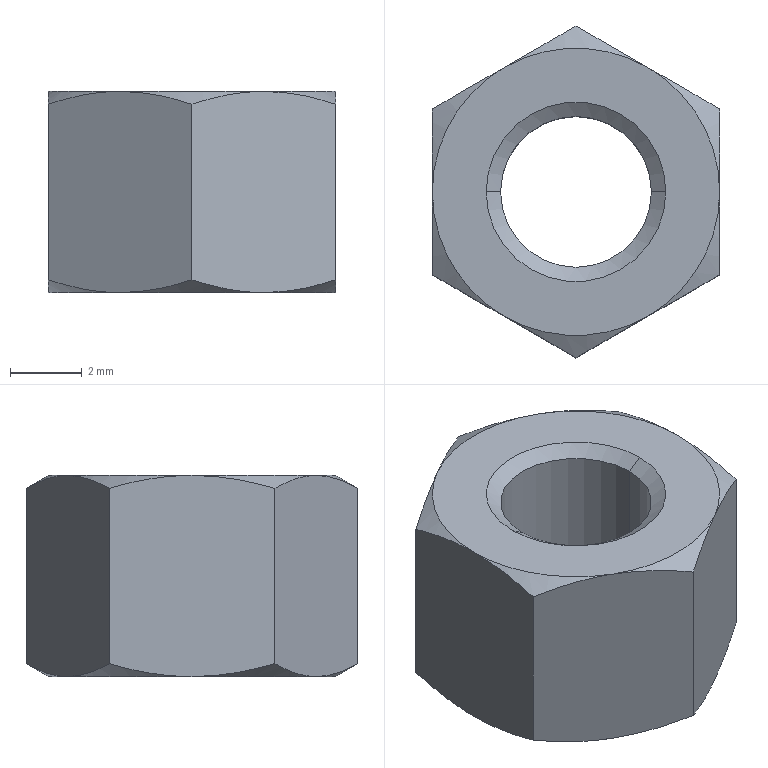Part | SolidWorks | features RevCut 3, Extrusion 1, LPattern 1 | 1 solid | 28 faces | box 8 x 9.238 x 5.6 mm | volume 229.964 mm3 | cone 16 | plane 8 | cylinder 4 | commonest cylinder face diameters 4.2 x2 5 x2
STEP:
#1=CARTESIAN_POINT('',(-2.5,0.,-5.6));
#2=VERTEX_POINT('',#1);
#3=CARTESIAN_POINT('',(2.5,0.,-5.6));
#4=VERTEX_POINT('',#3);
#5=CARTESIAN_POINT('',(0.,0.,-5.6));
#6=DIRECTION('',(0.,0.,1.));
#7=DIRECTION('',(-1.,0.,0.));
#8=AXIS2_PLACEMENT_3D('',#5,#6,#7);
#9=CIRCLE('',#8,2.5);
#10=EDGE_CURVE('',#2,#4,#9,.T.);
#11=ORIENTED_EDGE('',*,*,#10,.F.);
#12=CARTESIAN_POINT('',(-2.5,0.,-5.575));
#13=VERTEX_POINT('',#12);
#14=CARTESIAN_POINT('',(-2.5,0.,-25.038));
#15=DIRECTION('',(0.,0.,1.));
#16=VECTOR('',#15,1000.);
#17=LINE('',#14,#16);
#18=EDGE_CURVE('',#2,#13,#17,.T.);
#19=ORIENTED_EDGE('',*,*,#18,.T.);
#20=CARTESIAN_POINT('',(2.5,0.,-5.575));
#21=VERTEX_POINT('',#20);
#22=CARTESIAN_POINT('',(0.,0.,-5.575));
#23=DIRECTION('',(0.,0.,1.));
#24=DIRECTION('',(1.,0.,0.));
#25=AXIS2_PLACEMENT_3D('',#22,#23,#24);
#26=CIRCLE('',#25,2.5);
#27=EDGE_CURVE('',#13,#21,#26,.T.);
#28=ORIENTED_EDGE('',*,*,#27,.T.);
#29=CARTESIAN_POINT('',(2.5,0.,-25.038));
#30=DIRECTION('',(0.,0.,1.));
#31=VECTOR('',#30,1000.);
#32=LINE('',#29,#31);
#33=EDGE_CURVE('',#4,#21,#32,.T.);
#34=ORIENTED_EDGE('',*,*,#33,.F.);
#35=EDGE_LOOP('',(#11,#19,#28,#34));
#36=FACE_OUTER_BOUND('',#35,.T.);
#37=CARTESIAN_POINT('',(0.,0.,-25.038));
#38=DIRECTION('',(0.,0.,1.));
#39=DIRECTION('',(1.,0.,0.));
#40=AXIS2_PLACEMENT_3D('',#37,#38,#39);
#41=CYLINDRICAL_SURFACE('',#40,2.5);
#42=ADVANCED_FACE('',(#36),#41,.F.);
#43=CARTESIAN_POINT('',(-2.1,0.,-5.295));
#44=VERTEX_POINT('',#43);
#45=CARTESIAN_POINT('',(2.1,0.,-5.295));
#46=VERTEX_POINT('',#45);
#47=CARTESIAN_POINT('',(0.,0.,-5.295));
#48=DIRECTION('',(0.,0.,1.));
#49=DIRECTION('',(-1.,0.,0.));
#50=AXIS2_PLACEMENT_3D('',#47,#48,#49);
#51=CIRCLE('',#50,2.1);
#52=EDGE_CURVE('',#44,#46,#51,.T.);
#53=ORIENTED_EDGE('',*,*,#52,.T.);
#54=CARTESIAN_POINT('',(2.5,0.,-5.575));
#55=DIRECTION('',(0.8192,0.,-0.5736));
#56=VECTOR('',#55,1000.);
#57=LINE('',#54,#56);
#58=EDGE_CURVE('',#46,#21,#57,.T.);
#59=ORIENTED_EDGE('',*,*,#58,.T.);
#60=ORIENTED_EDGE('',*,*,#27,.F.);
#61=CARTESIAN_POINT('',(-2.5,0.,-5.575));
#62=DIRECTION('',(-0.8192,0.,-0.5736));
#63=VECTOR('',#62,1000.);
#64=LINE('',#61,#63);
#65=EDGE_CURVE('',#44,#13,#64,.T.);
#66=ORIENTED_EDGE('',*,*,#65,.F.);
#67=EDGE_LOOP('',(#53,#59,#60,#66));
#68=FACE_OUTER_BOUND('',#67,.T.);
#69=CARTESIAN_POINT('',(0.,0.,-5.575));
#70=DIRECTION('',(0.,0.,-1.));
#71=DIRECTION('',(-1.,0.,0.));
#72=AXIS2_PLACEMENT_3D('',#69,#70,#71);
#73=CONICAL_SURFACE('',#72,2.5,0.9599);
#74=ADVANCED_FACE('',(#68),#73,.F.);
#75=CARTESIAN_POINT('',(2.1,0.,-0.2801));
#76=VERTEX_POINT('',#75);
#77=CARTESIAN_POINT('',(-2.1,0.,-0.2801));
#78=VERTEX_POINT('',#77);
#79=CARTESIAN_POINT('',(0.,0.,-0.2801));
#80=DIRECTION('',(0.,0.,-1.));
#81=DIRECTION('',(1.,0.,0.));
#82=AXIS2_PLACEMENT_3D('',#79,#80,#81);
#83=CIRCLE('',#82,2.1);
#84=EDGE_CURVE('',#76,#78,#83,.T.);
#85=ORIENTED_EDGE('',*,*,#84,.T.);
#86=CARTESIAN_POINT('',(-2.5,0.,0.));
#87=VERTEX_POINT('',#86);
#88=CARTESIAN_POINT('',(-2.06,0.,-0.3081));
#89=DIRECTION('',(-0.8192,0.,0.5736));
#90=VECTOR('',#89,1000.);
#91=LINE('',#88,#90);
#92=EDGE_CURVE('',#78,#87,#91,.T.);
#93=ORIENTED_EDGE('',*,*,#92,.T.);
#94=CARTESIAN_POINT('',(2.5,0.,0.));
#95=VERTEX_POINT('',#94);
#96=CARTESIAN_POINT('',(0.,0.,0.));
#97=DIRECTION('',(0.,0.,1.));
#98=DIRECTION('',(1.,0.,0.));
#99=AXIS2_PLACEMENT_3D('',#96,#97,#98);
#100=CIRCLE('',#99,2.5);
#101=EDGE_CURVE('',#87,#95,#100,.T.);
#102=ORIENTED_EDGE('',*,*,#101,.T.);
#103=CARTESIAN_POINT('',(2.06,0.,-0.3081));
#104=DIRECTION('',(0.8192,0.,0.5736));
#105=VECTOR('',#104,1000.);
#106=LINE('',#103,#105);
#107=EDGE_CURVE('',#76,#95,#106,.T.);
#108=ORIENTED_EDGE('',*,*,#107,.F.);
#109=EDGE_LOOP('',(#85,#93,#102,#108));
#110=FACE_OUTER_BOUND('',#109,.T.);
#111=CARTESIAN_POINT('',(0.,0.,-0.3081));
#112=DIRECTION('',(0.,0.,1.));
#113=DIRECTION('',(1.,0.,0.));
#114=AXIS2_PLACEMENT_3D('',#111,#112,#113);
#115=CONICAL_SURFACE('',#114,2.06,0.9599);
#116=ADVANCED_FACE('',(#110),#115,.F.);
#117=ORIENTED_EDGE('',*,*,#52,.F.);
#118=CARTESIAN_POINT('',(-2.1,0.,-5.6));
#119=DIRECTION('',(0.,0.,1.));
#120=VECTOR('',#119,1000.);
#121=LINE('',#118,#120);
#122=EDGE_CURVE('',#44,#78,#121,.T.);
#123=ORIENTED_EDGE('',*,*,#122,.T.);
#124=ORIENTED_EDGE('',*,*,#84,.F.);
#125=CARTESIAN_POINT('',(2.1,0.,-5.6));
#126=DIRECTION('',(0.,0.,1.));
#127=VECTOR('',#126,1000.);
#128=LINE('',#125,#127);
#129=EDGE_CURVE('',#46,#76,#128,.T.);
#130=ORIENTED_EDGE('',*,*,#129,.F.);
#131=EDGE_LOOP('',(#117,#123,#124,#130));
#132=FACE_OUTER_BOUND('',#131,.T.);
#133=CARTESIAN_POINT('',(0.,0.,-5.6));
#134=DIRECTION('',(0.,0.,1.));
#135=DIRECTION('',(1.,0.,0.));
#136=AXIS2_PLACEMENT_3D('',#133,#134,#135);
#137=CYLINDRICAL_SURFACE('',#136,2.1);
#138=ADVANCED_FACE('',(#132),#137,.F.);
#139=ORIENTED_EDGE('',*,*,#122,.F.);
#140=CARTESIAN_POINT('',(0.,0.,-5.295));
#141=DIRECTION('',(0.,0.,1.));
#142=DIRECTION('',(-1.,0.,0.));
#143=AXIS2_PLACEMENT_3D('',#140,#141,#142);
#144=CIRCLE('',#143,2.1);
#145=EDGE_CURVE('',#46,#44,#144,.T.);
#146=ORIENTED_EDGE('',*,*,#145,.F.);
#147=ORIENTED_EDGE('',*,*,#129,.T.);
#148=CARTESIAN_POINT('',(0.,0.,-0.2801));
#149=DIRECTION('',(0.,0.,-1.));
#150=DIRECTION('',(1.,0.,0.));
#151=AXIS2_PLACEMENT_3D('',#148,#149,#150);
#152=CIRCLE('',#151,2.1);
#153=EDGE_CURVE('',#78,#76,#152,.T.);
#154=ORIENTED_EDGE('',*,*,#153,.F.);
#155=EDGE_LOOP('',(#139,#146,#147,#154));
#156=FACE_OUTER_BOUND('',#155,.T.);
#157=CARTESIAN_POINT('',(0.,0.,-5.6));
#158=DIRECTION('',(0.,0.,1.));
#159=DIRECTION('',(1.,0.,0.));
#160=AXIS2_PLACEMENT_3D('',#157,#158,#159);
#161=CYLINDRICAL_SURFACE('',#160,2.1);
#162=ADVANCED_FACE('',(#156),#161,.F.);
#163=CARTESIAN_POINT('',(-4.,2.309,-5.243));
#164=VERTEX_POINT('',#163);
#165=CARTESIAN_POINT('',(-4.,2.309,-0.3573));
#166=VERTEX_POINT('',#165);
#167=CARTESIAN_POINT('',(-4.,2.309,-5.6));
#168=DIRECTION('',(0.,0.,1.));
#169=VECTOR('',#168,1000.);
#170=LINE('',#167,#169);
#171=EDGE_CURVE('',#164,#166,#170,.T.);
#172=ORIENTED_EDGE('',*,*,#171,.T.);
#173=CARTESIAN_POINT('',(-2.,3.464,0.));
#174=VERTEX_POINT('',#173);
#175=CARTESIAN_POINT('',(-4.,2.309,-0.3573));
#176=CARTESIAN_POINT('',(-3.346,2.687,-0.1392));
#177=CARTESIAN_POINT('',(-2.681,3.071,0.));
#178=CARTESIAN_POINT('',(-2.,3.464,0.));
#179=B_SPLINE_CURVE_WITH_KNOTS('',3,(#175,#176,#177,#178),.UNSPECIFIED.,.F.,.F.,(4,4),(0.000000238,0.002337),.UNSPECIFIED.);
#180=EDGE_CURVE('',#166,#174,#179,.T.);
#181=ORIENTED_EDGE('',*,*,#180,.T.);
#182=CARTESIAN_POINT('',(0.,4.619,-0.3573));
#183=VERTEX_POINT('',#182);
#184=CARTESIAN_POINT('',(-2.,3.464,0.));
#185=CARTESIAN_POINT('',(-1.661,3.66,0.));
#186=CARTESIAN_POINT('',(-1.322,3.856,-0.03421));
#187=CARTESIAN_POINT('',(-0.6554,4.24,-0.1587));
#188=CARTESIAN_POINT('',(-0.3264,4.43,-0.2485));
#189=CARTESIAN_POINT('',(0.,4.619,-0.3573));
#190=B_SPLINE_CURVE_WITH_KNOTS('',3,(#184,#185,#186,#187,#188,#189),.UNSPECIFIED.,.F.,.F.,(4,2,4),(0.002337,0.003501,0.004665),.UNSPECIFIED.);
#191=EDGE_CURVE('',#174,#183,#190,.T.);
#192=ORIENTED_EDGE('',*,*,#191,.T.);
#193=CARTESIAN_POINT('',(0.,4.619,-5.243));
#194=VERTEX_POINT('',#193);
#195=CARTESIAN_POINT('',(0.,4.619,-5.6));
#196=DIRECTION('',(0.,0.,1.));
#197=VECTOR('',#196,1000.);
#198=LINE('',#195,#197);
#199=EDGE_CURVE('',#194,#183,#198,.T.);
#200=ORIENTED_EDGE('',*,*,#199,.F.);
#201=CARTESIAN_POINT('',(-2.,3.464,-5.6));
#202=VERTEX_POINT('',#201);
#203=CARTESIAN_POINT('',(-2.,3.464,-5.6));
#204=CARTESIAN_POINT('',(-1.661,3.66,-5.6));
#205=CARTESIAN_POINT('',(-1.322,3.856,-5.566));
#206=CARTESIAN_POINT('',(-0.6554,4.24,-5.441));
#207=CARTESIAN_POINT('',(-0.3264,4.43,-5.352));
#208=CARTESIAN_POINT('',(0.,4.619,-5.243));
#209=B_SPLINE_CURVE_WITH_KNOTS('',3,(#203,#204,#205,#206,#207,#208),.UNSPECIFIED.,.F.,.F.,(4,2,4),(0.002337,0.003501,0.004665),.UNSPECIFIED.);
#210=EDGE_CURVE('',#202,#194,#209,.T.);
#211=ORIENTED_EDGE('',*,*,#210,.F.);
#212=CARTESIAN_POINT('',(-4.,2.309,-5.243));
#213=CARTESIAN_POINT('',(-3.346,2.687,-5.461));
#214=CARTESIAN_POINT('',(-2.681,3.071,-5.6));
#215=CARTESIAN_POINT('',(-2.,3.464,-5.6));
#216=B_SPLINE_CURVE_WITH_KNOTS('',3,(#212,#213,#214,#215),.UNSPECIFIED.,.F.,.F.,(4,4),(0.000000238,0.002337),.UNSPECIFIED.);
#217=EDGE_CURVE('',#164,#202,#216,.T.);
#218=ORIENTED_EDGE('',*,*,#217,.F.);
#219=EDGE_LOOP('',(#172,#181,#192,#200,#211,#218));
#220=FACE_OUTER_BOUND('',#219,.T.);
#221=CARTESIAN_POINT('',(0.,4.619,-5.6));
#222=DIRECTION('',(-0.5,0.866,0.));
#223=DIRECTION('',(-0.866,-0.5,0.));
#224=AXIS2_PLACEMENT_3D('',#221,#222,#223);
#225=PLANE('',#224);
#226=ADVANCED_FACE('',(#220),#225,.T.);
#227=ORIENTED_EDGE('',*,*,#199,.T.);
#228=CARTESIAN_POINT('',(2.,3.464,0.));
#229=VERTEX_POINT('',#228);
#230=CARTESIAN_POINT('',(0.,4.619,-0.3573));
#231=CARTESIAN_POINT('',(0.6543,4.241,-0.1392));
#232=CARTESIAN_POINT('',(1.319,3.858,0.));
#233=CARTESIAN_POINT('',(2.,3.464,0.));
#234=B_SPLINE_CURVE_WITH_KNOTS('',3,(#230,#231,#232,#233),.UNSPECIFIED.,.F.,.F.,(4,4),(0.000000238,0.002337),.UNSPECIFIED.);
#235=EDGE_CURVE('',#183,#229,#234,.T.);
#236=ORIENTED_EDGE('',*,*,#235,.T.);
#237=CARTESIAN_POINT('',(4.,2.309,-0.3573));
#238=VERTEX_POINT('',#237);
#239=CARTESIAN_POINT('',(2.,3.464,0.));
#240=CARTESIAN_POINT('',(2.339,3.268,0.));
#241=CARTESIAN_POINT('',(2.678,3.072,-0.03421));
#242=CARTESIAN_POINT('',(3.345,2.688,-0.1587));
#243=CARTESIAN_POINT('',(3.674,2.498,-0.2485));
#244=CARTESIAN_POINT('',(4.,2.309,-0.3573));
#245=B_SPLINE_CURVE_WITH_KNOTS('',3,(#239,#240,#241,#242,#243,#244),.UNSPECIFIED.,.F.,.F.,(4,2,4),(0.002337,0.003501,0.004665),.UNSPECIFIED.);
#246=EDGE_CURVE('',#229,#238,#245,.T.);
#247=ORIENTED_EDGE('',*,*,#246,.T.);
#248=CARTESIAN_POINT('',(4.,2.309,-5.243));
#249=VERTEX_POINT('',#248);
#250=CARTESIAN_POINT('',(4.,2.309,-5.6));
#251=DIRECTION('',(0.,0.,1.));
#252=VECTOR('',#251,1000.);
#253=LINE('',#250,#252);
#254=EDGE_CURVE('',#249,#238,#253,.T.);
#255=ORIENTED_EDGE('',*,*,#254,.F.);
#256=CARTESIAN_POINT('',(2.,3.464,-5.6));
#257=VERTEX_POINT('',#256);
#258=CARTESIAN_POINT('',(2.,3.464,-5.6));
#259=CARTESIAN_POINT('',(2.339,3.268,-5.6));
#260=CARTESIAN_POINT('',(2.678,3.072,-5.566));
#261=CARTESIAN_POINT('',(3.345,2.688,-5.441));
#262=CARTESIAN_POINT('',(3.674,2.498,-5.352));
#263=CARTESIAN_POINT('',(4.,2.309,-5.243));
#264=B_SPLINE_CURVE_WITH_KNOTS('',3,(#258,#259,#260,#261,#262,#263),.UNSPECIFIED.,.F.,.F.,(4,2,4),(0.002337,0.003501,0.004665),.UNSPECIFIED.);
#265=EDGE_CURVE('',#257,#249,#264,.T.);
#266=ORIENTED_EDGE('',*,*,#265,.F.);
#267=CARTESIAN_POINT('',(0.,4.619,-5.243));
#268=CARTESIAN_POINT('',(0.6543,4.241,-5.461));
#269=CARTESIAN_POINT('',(1.319,3.858,-5.6));
#270=CARTESIAN_POINT('',(2.,3.464,-5.6));
#271=B_SPLINE_CURVE_WITH_KNOTS('',3,(#267,#268,#269,#270),.UNSPECIFIED.,.F.,.F.,(4,4),(0.000000238,0.002337),.UNSPECIFIED.);
#272=EDGE_CURVE('',#194,#257,#271,.T.);
#273=ORIENTED_EDGE('',*,*,#272,.F.);
#274=EDGE_LOOP('',(#227,#236,#247,#255,#266,#273));
#275=FACE_OUTER_BOUND('',#274,.T.);
#276=CARTESIAN_POINT('',(4.,2.309,-5.6));
#277=DIRECTION('',(0.5,0.866,0.));
#278=DIRECTION('',(-0.866,0.5,0.));
#279=AXIS2_PLACEMENT_3D('',#276,#277,#278);
#280=PLANE('',#279);
#281=ADVANCED_FACE('',(#275),#280,.T.);
#282=CARTESIAN_POINT('',(4.,-2.309,-0.3573));
#283=VERTEX_POINT('',#282);
#284=CARTESIAN_POINT('',(4.,0.,0.));
#285=VERTEX_POINT('',#284);
#286=CARTESIAN_POINT('',(4.,-2.309,-0.3573));
#287=CARTESIAN_POINT('',(4.,-1.934,-0.2488));
#288=CARTESIAN_POINT('',(4.,-1.549,-0.1579));
#289=CARTESIAN_POINT('',(4.,-0.778,-0.03354));
#290=CARTESIAN_POINT('',(4.,-0.3903,0.));
#291=CARTESIAN_POINT('',(4.,0.,0.));
#292=B_SPLINE_CURVE_WITH_KNOTS('',3,(#286,#287,#288,#289,#290,#291),.UNSPECIFIED.,.F.,.F.,(4,2,4),(0.00412,0.005288,0.006457),.UNSPECIFIED.);
#293=EDGE_CURVE('',#283,#285,#292,.T.);
#294=ORIENTED_EDGE('',*,*,#293,.F.);
#295=CARTESIAN_POINT('',(4.,-2.309,-5.243));
#296=VERTEX_POINT('',#295);
#297=CARTESIAN_POINT('',(4.,-2.309,-5.6));
#298=DIRECTION('',(0.,0.,1.));
#299=VECTOR('',#298,1000.);
#300=LINE('',#297,#299);
#301=EDGE_CURVE('',#296,#283,#300,.T.);
#302=ORIENTED_EDGE('',*,*,#301,.F.);
#303=CARTESIAN_POINT('',(4.,0.,-5.6));
#304=VERTEX_POINT('',#303);
#305=CARTESIAN_POINT('',(4.,-2.309,-5.243));
#306=CARTESIAN_POINT('',(4.,-1.934,-5.351));
#307=CARTESIAN_POINT('',(4.,-1.549,-5.442));
#308=CARTESIAN_POINT('',(4.,-0.778,-5.566));
#309=CARTESIAN_POINT('',(4.,-0.3903,-5.6));
#310=CARTESIAN_POINT('',(4.,0.,-5.6));
#311=B_SPLINE_CURVE_WITH_KNOTS('',3,(#305,#306,#307,#308,#309,#310),.UNSPECIFIED.,.F.,.F.,(4,2,4),(0.00412,0.005288,0.006457),.UNSPECIFIED.);
#312=EDGE_CURVE('',#296,#304,#311,.T.);
#313=ORIENTED_EDGE('',*,*,#312,.T.);
#314=CARTESIAN_POINT('',(4.,0.,-5.6));
#315=CARTESIAN_POINT('',(4.,0.3905,-5.6));
#316=CARTESIAN_POINT('',(4.,0.7863,-5.566));
#317=CARTESIAN_POINT('',(4.,1.558,-5.44));
#318=CARTESIAN_POINT('',(4.,1.936,-5.351));
#319=CARTESIAN_POINT('',(4.,2.309,-5.243));
#320=B_SPLINE_CURVE_WITH_KNOTS('',3,(#314,#315,#316,#317,#318,#319),.UNSPECIFIED.,.F.,.F.,(4,2,4),(0.006457,0.007625,0.008794),.UNSPECIFIED.);
#321=EDGE_CURVE('',#304,#249,#320,.T.);
#322=ORIENTED_EDGE('',*,*,#321,.T.);
#323=ORIENTED_EDGE('',*,*,#254,.T.);
#324=CARTESIAN_POINT('',(4.,0.,0.));
#325=CARTESIAN_POINT('',(4.,0.3905,0.));
#326=CARTESIAN_POINT('',(4.,0.7863,-0.03447));
#327=CARTESIAN_POINT('',(4.,1.558,-0.1597));
#328=CARTESIAN_POINT('',(4.,1.936,-0.2495));
#329=CARTESIAN_POINT('',(4.,2.309,-0.3573));
#330=B_SPLINE_CURVE_WITH_KNOTS('',3,(#324,#325,#326,#327,#328,#329),.UNSPECIFIED.,.F.,.F.,(4,2,4),(0.006457,0.007625,0.008794),.UNSPECIFIED.);
#331=EDGE_CURVE('',#285,#238,#330,.T.);
#332=ORIENTED_EDGE('',*,*,#331,.F.);
#333=EDGE_LOOP('',(#294,#302,#313,#322,#323,#332));
#334=FACE_OUTER_BOUND('',#333,.T.);
#335=CARTESIAN_POINT('',(4.,2.309,-5.6));
#336=DIRECTION('',(-1.,0.,0.));
#337=DIRECTION('',(0.,0.,1.));
#338=AXIS2_PLACEMENT_3D('',#335,#336,#337);
#339=PLANE('',#338);
#340=ADVANCED_FACE('',(#334),#339,.F.);
#341=ORIENTED_EDGE('',*,*,#301,.T.);
#342=CARTESIAN_POINT('',(2.,-3.464,0.));
#343=VERTEX_POINT('',#342);
#344=CARTESIAN_POINT('',(4.,-2.309,-0.3573));
#345=CARTESIAN_POINT('',(3.346,-2.687,-0.1392));
#346=CARTESIAN_POINT('',(2.681,-3.071,0.));
#347=CARTESIAN_POINT('',(2.,-3.464,0.));
#348=B_SPLINE_CURVE_WITH_KNOTS('',3,(#344,#345,#346,#347),.UNSPECIFIED.,.F.,.F.,(4,4),(0.000000238,0.002337),.UNSPECIFIED.);
#349=EDGE_CURVE('',#283,#343,#348,.T.);
#350=ORIENTED_EDGE('',*,*,#349,.T.);
#351=CARTESIAN_POINT('',(0.,-4.619,-0.3573));
#352=VERTEX_POINT('',#351);
#353=CARTESIAN_POINT('',(2.,-3.464,0.));
#354=CARTESIAN_POINT('',(1.661,-3.66,0.));
#355=CARTESIAN_POINT('',(1.322,-3.856,-0.03421));
#356=CARTESIAN_POINT('',(0.6554,-4.24,-0.1587));
#357=CARTESIAN_POINT('',(0.3264,-4.43,-0.2485));
#358=CARTESIAN_POINT('',(0.,-4.619,-0.3573));
#359=B_SPLINE_CURVE_WITH_KNOTS('',3,(#353,#354,#355,#356,#357,#358),.UNSPECIFIED.,.F.,.F.,(4,2,4),(0.002337,0.003501,0.004665),.UNSPECIFIED.);
#360=EDGE_CURVE('',#343,#352,#359,.T.);
#361=ORIENTED_EDGE('',*,*,#360,.T.);
#362=CARTESIAN_POINT('',(0.,-4.619,-5.243));
#363=VERTEX_POINT('',#362);
#364=CARTESIAN_POINT('',(0.,-4.619,-5.6));
#365=DIRECTION('',(0.,0.,1.));
#366=VECTOR('',#365,1000.);
#367=LINE('',#364,#366);
#368=EDGE_CURVE('',#363,#352,#367,.T.);
#369=ORIENTED_EDGE('',*,*,#368,.F.);
#370=CARTESIAN_POINT('',(2.,-3.464,-5.6));
#371=VERTEX_POINT('',#370);
#372=CARTESIAN_POINT('',(2.,-3.464,-5.6));
#373=CARTESIAN_POINT('',(1.661,-3.66,-5.6));
#374=CARTESIAN_POINT('',(1.322,-3.856,-5.566));
#375=CARTESIAN_POINT('',(0.6554,-4.24,-5.441));
#376=CARTESIAN_POINT('',(0.3264,-4.43,-5.352));
#377=CARTESIAN_POINT('',(0.,-4.619,-5.243));
#378=B_SPLINE_CURVE_WITH_KNOTS('',3,(#372,#373,#374,#375,#376,#377),.UNSPECIFIED.,.F.,.F.,(4,2,4),(0.002337,0.003501,0.004665),.UNSPECIFIED.);
#379=EDGE_CURVE('',#371,#363,#378,.T.);
#380=ORIENTED_EDGE('',*,*,#379,.F.);
#381=CARTESIAN_POINT('',(4.,-2.309,-5.243));
#382=CARTESIAN_POINT('',(3.346,-2.687,-5.461));
#383=CARTESIAN_POINT('',(2.681,-3.071,-5.6));
#384=CARTESIAN_POINT('',(2.,-3.464,-5.6));
#385=B_SPLINE_CURVE_WITH_KNOTS('',3,(#381,#382,#383,#384),.UNSPECIFIED.,.F.,.F.,(4,4),(0.000000238,0.002337),.UNSPECIFIED.);
#386=EDGE_CURVE('',#296,#371,#385,.T.);
#387=ORIENTED_EDGE('',*,*,#386,.F.);
#388=EDGE_LOOP('',(#341,#350,#361,#369,#380,#387));
#389=FACE_OUTER_BOUND('',#388,.T.);
#390=CARTESIAN_POINT('',(0.,-4.619,-5.6));
#391=DIRECTION('',(0.5,-0.866,0.));
#392=DIRECTION('',(0.866,0.5,0.));
#393=AXIS2_PLACEMENT_3D('',#390,#391,#392);
#394=PLANE('',#393);
#395=ADVANCED_FACE('',(#389),#394,.T.);
#396=ORIENTED_EDGE('',*,*,#368,.T.);
#397=CARTESIAN_POINT('',(-2.,-3.464,0.));
#398=VERTEX_POINT('',#397);
#399=CARTESIAN_POINT('',(0.,-4.619,-0.3573));
#400=CARTESIAN_POINT('',(-0.6543,-4.241,-0.1392));
#401=CARTESIAN_POINT('',(-1.319,-3.858,0.));
#402=CARTESIAN_POINT('',(-2.,-3.464,0.));
#403=B_SPLINE_CURVE_WITH_KNOTS('',3,(#399,#400,#401,#402),.UNSPECIFIED.,.F.,.F.,(4,4),(0.000000238,0.002337),.UNSPECIFIED.);
#404=EDGE_CURVE('',#352,#398,#403,.T.);
#405=ORIENTED_EDGE('',*,*,#404,.T.);
#406=CARTESIAN_POINT('',(-4.,-2.309,-0.3573));
#407=VERTEX_POINT('',#406);
#408=CARTESIAN_POINT('',(-2.,-3.464,0.));
#409=CARTESIAN_POINT('',(-2.339,-3.268,0.));
#410=CARTESIAN_POINT('',(-2.678,-3.072,-0.03421));
#411=CARTESIAN_POINT('',(-3.345,-2.688,-0.1587));
#412=CARTESIAN_POINT('',(-3.674,-2.498,-0.2485));
#413=CARTESIAN_POINT('',(-4.,-2.309,-0.3573));
#414=B_SPLINE_CURVE_WITH_KNOTS('',3,(#408,#409,#410,#411,#412,#413),.UNSPECIFIED.,.F.,.F.,(4,2,4),(0.002337,0.003501,0.004665),.UNSPECIFIED.);
#415=EDGE_CURVE('',#398,#407,#414,.T.);
#416=ORIENTED_EDGE('',*,*,#415,.T.);
#417=CARTESIAN_POINT('',(-4.,-2.309,-5.243));
#418=VERTEX_POINT('',#417);
#419=CARTESIAN_POINT('',(-4.,-2.309,-5.6));
#420=DIRECTION('',(0.,0.,1.));
#421=VECTOR('',#420,1000.);
#422=LINE('',#419,#421);
#423=EDGE_CURVE('',#418,#407,#422,.T.);
#424=ORIENTED_EDGE('',*,*,#423,.F.);
#425=CARTESIAN_POINT('',(-2.,-3.464,-5.6));
#426=VERTEX_POINT('',#425);
#427=CARTESIAN_POINT('',(-2.,-3.464,-5.6));
#428=CARTESIAN_POINT('',(-2.339,-3.268,-5.6));
#429=CARTESIAN_POINT('',(-2.678,-3.072,-5.566));
#430=CARTESIAN_POINT('',(-3.345,-2.688,-5.441));
#431=CARTESIAN_POINT('',(-3.674,-2.498,-5.352));
#432=CARTESIAN_POINT('',(-4.,-2.309,-5.243));
#433=B_SPLINE_CURVE_WITH_KNOTS('',3,(#427,#428,#429,#430,#431,#432),.UNSPECIFIED.,.F.,.F.,(4,2,4),(0.002337,0.003501,0.004665),.UNSPECIFIED.);
#434=EDGE_CURVE('',#426,#418,#433,.T.);
#435=ORIENTED_EDGE('',*,*,#434,.F.);
#436=CARTESIAN_POINT('',(0.,-4.619,-5.243));
#437=CARTESIAN_POINT('',(-0.6543,-4.241,-5.461));
#438=CARTESIAN_POINT('',(-1.319,-3.858,-5.6));
#439=CARTESIAN_POINT('',(-2.,-3.464,-5.6));
#440=B_SPLINE_CURVE_WITH_KNOTS('',3,(#436,#437,#438,#439),.UNSPECIFIED.,.F.,.F.,(4,4),(0.000000238,0.002337),.UNSPECIFIED.);
#441=EDGE_CURVE('',#363,#426,#440,.T.);
#442=ORIENTED_EDGE('',*,*,#441,.F.);
#443=EDGE_LOOP('',(#396,#405,#416,#424,#435,#442));
#444=FACE_OUTER_BOUND('',#443,.T.);
#445=CARTESIAN_POINT('',(-4.,-2.309,-5.6));
#446=DIRECTION('',(-0.5,-0.866,0.));
#447=DIRECTION('',(0.866,-0.5,0.));
#448=AXIS2_PLACEMENT_3D('',#445,#446,#447);
#449=PLANE('',#448);
#450=ADVANCED_FACE('',(#444),#449,.T.);
#451=ORIENTED_EDGE('',*,*,#423,.T.);
#452=CARTESIAN_POINT('',(-4.,0.,0.));
#453=VERTEX_POINT('',#452);
#454=CARTESIAN_POINT('',(-4.,-2.309,-0.3573));
#455=CARTESIAN_POINT('',(-4.,-1.934,-0.2488));
#456=CARTESIAN_POINT('',(-4.,-1.549,-0.1579));
#457=CARTESIAN_POINT('',(-4.,-0.778,-0.03354));
#458=CARTESIAN_POINT('',(-4.,-0.3903,0.));
#459=CARTESIAN_POINT('',(-4.,0.,0.));
#460=B_SPLINE_CURVE_WITH_KNOTS('',3,(#454,#455,#456,#457,#458,#459),.UNSPECIFIED.,.F.,.F.,(4,2,4),(0.00412,0.005288,0.006457),.UNSPECIFIED.);
#461=EDGE_CURVE('',#407,#453,#460,.T.);
#462=ORIENTED_EDGE('',*,*,#461,.T.);
#463=CARTESIAN_POINT('',(-4.,0.,0.));
#464=CARTESIAN_POINT('',(-4.,0.3905,0.));
#465=CARTESIAN_POINT('',(-4.,0.7863,-0.03447));
#466=CARTESIAN_POINT('',(-4.,1.558,-0.1597));
#467=CARTESIAN_POINT('',(-4.,1.936,-0.2495));
#468=CARTESIAN_POINT('',(-4.,2.309,-0.3573));
#469=B_SPLINE_CURVE_WITH_KNOTS('',3,(#463,#464,#465,#466,#467,#468),.UNSPECIFIED.,.F.,.F.,(4,2,4),(0.006457,0.007625,0.008794),.UNSPECIFIED.);
#470=EDGE_CURVE('',#453,#166,#469,.T.);
#471=ORIENTED_EDGE('',*,*,#470,.T.);
#472=ORIENTED_EDGE('',*,*,#171,.F.);
#473=CARTESIAN_POINT('',(-4.,0.,-5.6));
#474=VERTEX_POINT('',#473);
#475=CARTESIAN_POINT('',(-4.,0.,-5.6));
#476=CARTESIAN_POINT('',(-4.,0.3905,-5.6));
#477=CARTESIAN_POINT('',(-4.,0.7863,-5.566));
#478=CARTESIAN_POINT('',(-4.,1.558,-5.44));
#479=CARTESIAN_POINT('',(-4.,1.936,-5.351));
#480=CARTESIAN_POINT('',(-4.,2.309,-5.243));
#481=B_SPLINE_CURVE_WITH_KNOTS('',3,(#475,#476,#477,#478,#479,#480),.UNSPECIFIED.,.F.,.F.,(4,2,4),(0.006457,0.007625,0.008794),.UNSPECIFIED.);
#482=EDGE_CURVE('',#474,#164,#481,.T.);
#483=ORIENTED_EDGE('',*,*,#482,.F.);
#484=CARTESIAN_POINT('',(-4.,-2.309,-5.243));
#485=CARTESIAN_POINT('',(-4.,-1.934,-5.351));
#486=CARTESIAN_POINT('',(-4.,-1.549,-5.442));
#487=CARTESIAN_POINT('',(-4.,-0.778,-5.566));
#488=CARTESIAN_POINT('',(-4.,-0.3903,-5.6));
#489=CARTESIAN_POINT('',(-4.,0.,-5.6));
#490=B_SPLINE_CURVE_WITH_KNOTS('',3,(#484,#485,#486,#487,#488,#489),.UNSPECIFIED.,.F.,.F.,(4,2,4),(0.00412,0.005288,0.006457),.UNSPECIFIED.);
#491=EDGE_CURVE('',#418,#474,#490,.T.);
#492=ORIENTED_EDGE('',*,*,#491,.F.);
#493=EDGE_LOOP('',(#451,#462,#471,#472,#483,#492));
#494=FACE_OUTER_BOUND('',#493,.T.);
#495=CARTESIAN_POINT('',(-4.,2.309,-5.6));
#496=DIRECTION('',(-1.,0.,0.));
#497=DIRECTION('',(0.,0.,1.));
#498=AXIS2_PLACEMENT_3D('',#495,#496,#497);
#499=PLANE('',#498);
#500=ADVANCED_FACE('',(#494),#499,.T.);
#501=CARTESIAN_POINT('',(0.,0.,0.));
#502=DIRECTION('',(0.,0.,1.));
#503=DIRECTION('',(1.,0.,0.));
#504=AXIS2_PLACEMENT_3D('',#501,#502,#503);
#505=CIRCLE('',#504,2.5);
#506=EDGE_CURVE('',#95,#87,#505,.T.);
#507=ORIENTED_EDGE('',*,*,#506,.F.);
#508=ORIENTED_EDGE('',*,*,#101,.F.);
#509=EDGE_LOOP('',(#507,#508));
#510=FACE_BOUND('',#509,.T.);
#511=CARTESIAN_POINT('',(0.,0.,0.));
#512=DIRECTION('',(0.,0.,-1.));
#513=DIRECTION('',(-1.,0.,0.));
#514=AXIS2_PLACEMENT_3D('',#511,#512,#513);
#515=CIRCLE('',#514,4.);
#516=EDGE_CURVE('',#453,#174,#515,.T.);
#517=ORIENTED_EDGE('',*,*,#516,.F.);
#518=CARTESIAN_POINT('',(0.,0.,0.));
#519=DIRECTION('',(0.,0.,-1.));
#520=DIRECTION('',(-1.,0.,0.));
#521=AXIS2_PLACEMENT_3D('',#518,#519,#520);
#522=CIRCLE('',#521,4.);
#523=EDGE_CURVE('',#398,#453,#522,.T.);
#524=ORIENTED_EDGE('',*,*,#523,.F.);
#525=CARTESIAN_POINT('',(0.,0.,0.));
#526=DIRECTION('',(0.,0.,-1.));
#527=DIRECTION('',(-1.,0.,0.));
#528=AXIS2_PLACEMENT_3D('',#525,#526,#527);
#529=CIRCLE('',#528,4.);
#530=EDGE_CURVE('',#343,#398,#529,.T.);
#531=ORIENTED_EDGE('',*,*,#530,.F.);
#532=CARTESIAN_POINT('',(0.,0.,0.));
#533=DIRECTION('',(0.,0.,-1.));
#534=DIRECTION('',(-1.,0.,0.));
#535=AXIS2_PLACEMENT_3D('',#532,#533,#534);
#536=CIRCLE('',#535,4.);
#537=EDGE_CURVE('',#285,#343,#536,.T.);
#538=ORIENTED_EDGE('',*,*,#537,.F.);
#539=CARTESIAN_POINT('',(0.,0.,0.));
#540=DIRECTION('',(0.,0.,1.));
#541=DIRECTION('',(1.,0.,0.));
#542=AXIS2_PLACEMENT_3D('',#539,#540,#541);
#543=CIRCLE('',#542,4.);
#544=EDGE_CURVE('',#285,#229,#543,.T.);
#545=ORIENTED_EDGE('',*,*,#544,.T.);
#546=CARTESIAN_POINT('',(0.,0.,0.));
#547=DIRECTION('',(0.,0.,-1.));
#548=DIRECTION('',(-1.,0.,0.));
#549=AXIS2_PLACEMENT_3D('',#546,#547,#548);
#550=CIRCLE('',#549,4.);
#551=EDGE_CURVE('',#174,#229,#550,.T.);
#552=ORIENTED_EDGE('',*,*,#551,.F.);
#553=EDGE_LOOP('',(#517,#524,#531,#538,#545,#552));
#554=FACE_OUTER_BOUND('',#553,.T.);
#555=CARTESIAN_POINT('',(0.,4.619,0.));
#556=DIRECTION('',(0.,0.,-1.));
#557=DIRECTION('',(-1.,0.,0.));
#558=AXIS2_PLACEMENT_3D('',#555,#556,#557);
#559=PLANE('',#558);
#560=ADVANCED_FACE('',(#510,#554),#559,.F.);
#561=CARTESIAN_POINT('',(0.,0.,-5.6));
#562=DIRECTION('',(0.,0.,1.));
#563=DIRECTION('',(-1.,0.,0.));
#564=AXIS2_PLACEMENT_3D('',#561,#562,#563);
#565=CIRCLE('',#564,2.5);
#566=EDGE_CURVE('',#4,#2,#565,.T.);
#567=ORIENTED_EDGE('',*,*,#566,.T.);
#568=ORIENTED_EDGE('',*,*,#10,.T.);
#569=EDGE_LOOP('',(#567,#568));
#570=FACE_BOUND('',#569,.T.);
#571=CARTESIAN_POINT('',(0.,0.,-5.6));
#572=DIRECTION('',(0.,0.,1.));
#573=DIRECTION('',(-1.,0.,0.));
#574=AXIS2_PLACEMENT_3D('',#571,#572,#573);
#575=CIRCLE('',#574,4.);
#576=EDGE_CURVE('',#474,#426,#575,.T.);
#577=ORIENTED_EDGE('',*,*,#576,.F.);
#578=CARTESIAN_POINT('',(0.,0.,-5.6));
#579=DIRECTION('',(0.,0.,1.));
#580=DIRECTION('',(-1.,0.,0.));
#581=AXIS2_PLACEMENT_3D('',#578,#579,#580);
#582=CIRCLE('',#581,4.);
#583=EDGE_CURVE('',#202,#474,#582,.T.);
#584=ORIENTED_EDGE('',*,*,#583,.F.);
#585=CARTESIAN_POINT('',(0.,0.,-5.6));
#586=DIRECTION('',(0.,0.,1.));
#587=DIRECTION('',(-1.,0.,0.));
#588=AXIS2_PLACEMENT_3D('',#585,#586,#587);
#589=CIRCLE('',#588,4.);
#590=EDGE_CURVE('',#257,#202,#589,.T.);
#591=ORIENTED_EDGE('',*,*,#590,.F.);
#592=CARTESIAN_POINT('',(0.,0.,-5.6));
#593=DIRECTION('',(0.,0.,1.));
#594=DIRECTION('',(1.,0.,0.));
#595=AXIS2_PLACEMENT_3D('',#592,#593,#594);
#596=CIRCLE('',#595,4.);
#597=EDGE_CURVE('',#304,#257,#596,.T.);
#598=ORIENTED_EDGE('',*,*,#597,.F.);
#599=CARTESIAN_POINT('',(0.,0.,-5.6));
#600=DIRECTION('',(0.,0.,1.));
#601=DIRECTION('',(-1.,0.,0.));
#602=AXIS2_PLACEMENT_3D('',#599,#600,#601);
#603=CIRCLE('',#602,4.);
#604=EDGE_CURVE('',#371,#304,#603,.T.);
#605=ORIENTED_EDGE('',*,*,#604,.F.);
#606=CARTESIAN_POINT('',(0.,0.,-5.6));
#607=DIRECTION('',(0.,0.,1.));
#608=DIRECTION('',(-1.,0.,0.));
#609=AXIS2_PLACEMENT_3D('',#606,#607,#608);
#610=CIRCLE('',#609,4.);
#611=EDGE_CURVE('',#426,#371,#610,.T.);
#612=ORIENTED_EDGE('',*,*,#611,.F.);
#613=EDGE_LOOP('',(#577,#584,#591,#598,#605,#612));
#614=FACE_OUTER_BOUND('',#613,.T.);
#615=CARTESIAN_POINT('',(0.,4.619,-5.6));
#616=DIRECTION('',(0.,0.,-1.));
#617=DIRECTION('',(-1.,0.,0.));
#618=AXIS2_PLACEMENT_3D('',#615,#616,#617);
#619=PLANE('',#618);
#620=ADVANCED_FACE('',(#570,#614),#619,.T.);
#621=ORIENTED_EDGE('',*,*,#217,.T.);
#622=ORIENTED_EDGE('',*,*,#583,.T.);
#623=ORIENTED_EDGE('',*,*,#482,.T.);
#624=EDGE_LOOP('',(#621,#622,#623));
#625=FACE_OUTER_BOUND('',#624,.T.);
#626=CARTESIAN_POINT('',(0.,0.,-5.6));
#627=DIRECTION('',(0.,0.,1.));
#628=DIRECTION('',(1.,0.,0.));
#629=AXIS2_PLACEMENT_3D('',#626,#627,#628);
#630=CONICAL_SURFACE('',#629,4.,1.047);
#631=ADVANCED_FACE('',(#625),#630,.T.);
#632=ORIENTED_EDGE('',*,*,#210,.T.);
#633=ORIENTED_EDGE('',*,*,#272,.T.);
#634=ORIENTED_EDGE('',*,*,#590,.T.);
#635=EDGE_LOOP('',(#632,#633,#634));
#636=FACE_OUTER_BOUND('',#635,.T.);
#637=CARTESIAN_POINT('',(0.,0.,-5.6));
#638=DIRECTION('',(0.,0.,1.));
#639=DIRECTION('',(1.,0.,0.));
#640=AXIS2_PLACEMENT_3D('',#637,#638,#639);
#641=CONICAL_SURFACE('',#640,4.,1.047);
#642=ADVANCED_FACE('',(#636),#641,.T.);
#643=ORIENTED_EDGE('',*,*,#265,.T.);
#644=ORIENTED_EDGE('',*,*,#321,.F.);
#645=ORIENTED_EDGE('',*,*,#597,.T.);
#646=EDGE_LOOP('',(#643,#644,#645));
#647=FACE_OUTER_BOUND('',#646,.T.);
#648=CARTESIAN_POINT('',(0.,0.,-5.6));
#649=DIRECTION('',(0.,0.,1.));
#650=DIRECTION('',(1.,0.,0.));
#651=AXIS2_PLACEMENT_3D('',#648,#649,#650);
#652=CONICAL_SURFACE('',#651,4.,1.047);
#653=ADVANCED_FACE('',(#647),#652,.T.);
#654=ORIENTED_EDGE('',*,*,#386,.T.);
#655=ORIENTED_EDGE('',*,*,#604,.T.);
#656=ORIENTED_EDGE('',*,*,#312,.F.);
#657=EDGE_LOOP('',(#654,#655,#656));
#658=FACE_OUTER_BOUND('',#657,.T.);
#659=CARTESIAN_POINT('',(0.,0.,-5.6));
#660=DIRECTION('',(0.,0.,1.));
#661=DIRECTION('',(1.,0.,0.));
#662=AXIS2_PLACEMENT_3D('',#659,#660,#661);
#663=CONICAL_SURFACE('',#662,4.,1.047);
#664=ADVANCED_FACE('',(#658),#663,.T.);
#665=ORIENTED_EDGE('',*,*,#379,.T.);
#666=ORIENTED_EDGE('',*,*,#441,.T.);
#667=ORIENTED_EDGE('',*,*,#611,.T.);
#668=EDGE_LOOP('',(#665,#666,#667));
#669=FACE_OUTER_BOUND('',#668,.T.);
#670=CARTESIAN_POINT('',(0.,0.,-5.6));
#671=DIRECTION('',(0.,0.,1.));
#672=DIRECTION('',(1.,0.,0.));
#673=AXIS2_PLACEMENT_3D('',#670,#671,#672);
#674=CONICAL_SURFACE('',#673,4.,1.047);
#675=ADVANCED_FACE('',(#669),#674,.T.);
#676=ORIENTED_EDGE('',*,*,#434,.T.);
#677=ORIENTED_EDGE('',*,*,#491,.T.);
#678=ORIENTED_EDGE('',*,*,#576,.T.);
#679=EDGE_LOOP('',(#676,#677,#678));
#680=FACE_OUTER_BOUND('',#679,.T.);
#681=CARTESIAN_POINT('',(0.,0.,-5.6));
#682=DIRECTION('',(0.,0.,1.));
#683=DIRECTION('',(1.,0.,0.));
#684=AXIS2_PLACEMENT_3D('',#681,#682,#683);
#685=CONICAL_SURFACE('',#684,4.,1.047);
#686=ADVANCED_FACE('',(#680),#685,.T.);
#687=ORIENTED_EDGE('',*,*,#523,.T.);
#688=ORIENTED_EDGE('',*,*,#461,.F.);
#689=ORIENTED_EDGE('',*,*,#415,.F.);
#690=EDGE_LOOP('',(#687,#688,#689));
#691=FACE_OUTER_BOUND('',#690,.T.);
#692=CARTESIAN_POINT('',(0.,0.,0.));
#693=DIRECTION('',(0.,0.,-1.));
#694=DIRECTION('',(-1.,0.,0.));
#695=AXIS2_PLACEMENT_3D('',#692,#693,#694);
#696=CONICAL_SURFACE('',#695,4.,1.047);
#697=ADVANCED_FACE('',(#691),#696,.T.);
#698=ORIENTED_EDGE('',*,*,#530,.T.);
#699=ORIENTED_EDGE('',*,*,#404,.F.);
#700=ORIENTED_EDGE('',*,*,#360,.F.);
#701=EDGE_LOOP('',(#698,#699,#700));
#702=FACE_OUTER_BOUND('',#701,.T.);
#703=CARTESIAN_POINT('',(0.,0.,0.));
#704=DIRECTION('',(0.,0.,-1.));
#705=DIRECTION('',(-1.,0.,0.));
#706=AXIS2_PLACEMENT_3D('',#703,#704,#705);
#707=CONICAL_SURFACE('',#706,4.,1.047);
#708=ADVANCED_FACE('',(#702),#707,.T.);
#709=ORIENTED_EDGE('',*,*,#293,.T.);
#710=ORIENTED_EDGE('',*,*,#537,.T.);
#711=ORIENTED_EDGE('',*,*,#349,.F.);
#712=EDGE_LOOP('',(#709,#710,#711));
#713=FACE_OUTER_BOUND('',#712,.T.);
#714=CARTESIAN_POINT('',(0.,0.,0.));
#715=DIRECTION('',(0.,0.,-1.));
#716=DIRECTION('',(-1.,0.,0.));
#717=AXIS2_PLACEMENT_3D('',#714,#715,#716);
#718=CONICAL_SURFACE('',#717,4.,1.047);
#719=ADVANCED_FACE('',(#713),#718,.T.);
#720=ORIENTED_EDGE('',*,*,#544,.F.);
#721=ORIENTED_EDGE('',*,*,#331,.T.);
#722=ORIENTED_EDGE('',*,*,#246,.F.);
#723=EDGE_LOOP('',(#720,#721,#722));
#724=FACE_OUTER_BOUND('',#723,.T.);
#725=CARTESIAN_POINT('',(0.,0.,0.));
#726=DIRECTION('',(0.,0.,-1.));
#727=DIRECTION('',(-1.,0.,0.));
#728=AXIS2_PLACEMENT_3D('',#725,#726,#727);
#729=CONICAL_SURFACE('',#728,4.,1.047);
#730=ADVANCED_FACE('',(#724),#729,.T.);
#731=ORIENTED_EDGE('',*,*,#551,.T.);
#732=ORIENTED_EDGE('',*,*,#235,.F.);
#733=ORIENTED_EDGE('',*,*,#191,.F.);
#734=EDGE_LOOP('',(#731,#732,#733));
#735=FACE_OUTER_BOUND('',#734,.T.);
#736=CARTESIAN_POINT('',(0.,0.,0.));
#737=DIRECTION('',(0.,0.,-1.));
#738=DIRECTION('',(-1.,0.,0.));
#739=AXIS2_PLACEMENT_3D('',#736,#737,#738);
#740=CONICAL_SURFACE('',#739,4.,1.047);
#741=ADVANCED_FACE('',(#735),#740,.T.);
#742=ORIENTED_EDGE('',*,*,#470,.F.);
#743=ORIENTED_EDGE('',*,*,#516,.T.);
#744=ORIENTED_EDGE('',*,*,#180,.F.);
#745=EDGE_LOOP('',(#742,#743,#744));
#746=FACE_OUTER_BOUND('',#745,.T.);
#747=CARTESIAN_POINT('',(0.,0.,0.));
#748=DIRECTION('',(0.,0.,-1.));
#749=DIRECTION('',(-1.,0.,0.));
#750=AXIS2_PLACEMENT_3D('',#747,#748,#749);
#751=CONICAL_SURFACE('',#750,4.,1.047);
#752=ADVANCED_FACE('',(#746),#751,.T.);
#753=ORIENTED_EDGE('',*,*,#92,.F.);
#754=ORIENTED_EDGE('',*,*,#153,.T.);
#755=ORIENTED_EDGE('',*,*,#107,.T.);
#756=ORIENTED_EDGE('',*,*,#506,.T.);
#757=EDGE_LOOP('',(#753,#754,#755,#756));
#758=FACE_OUTER_BOUND('',#757,.T.);
#759=CARTESIAN_POINT('',(0.,0.,-0.3081));
#760=DIRECTION('',(0.,0.,1.));
#761=DIRECTION('',(1.,0.,0.));
#762=AXIS2_PLACEMENT_3D('',#759,#760,#761);
#763=CONICAL_SURFACE('',#762,2.06,0.9599);
#764=ADVANCED_FACE('',(#758),#763,.F.);
#765=ORIENTED_EDGE('',*,*,#58,.F.);
#766=ORIENTED_EDGE('',*,*,#145,.T.);
#767=ORIENTED_EDGE('',*,*,#65,.T.);
#768=CARTESIAN_POINT('',(0.,0.,-5.575));
#769=DIRECTION('',(0.,0.,1.));
#770=DIRECTION('',(1.,0.,0.));
#771=AXIS2_PLACEMENT_3D('',#768,#769,#770);
#772=CIRCLE('',#771,2.5);
#773=EDGE_CURVE('',#21,#13,#772,.T.);
#774=ORIENTED_EDGE('',*,*,#773,.F.);
#775=EDGE_LOOP('',(#765,#766,#767,#774));
#776=FACE_OUTER_BOUND('',#775,.T.);
#777=CARTESIAN_POINT('',(0.,0.,-5.575));
#778=DIRECTION('',(0.,0.,-1.));
#779=DIRECTION('',(-1.,0.,0.));
#780=AXIS2_PLACEMENT_3D('',#777,#778,#779);
#781=CONICAL_SURFACE('',#780,2.5,0.9599);
#782=ADVANCED_FACE('',(#776),#781,.F.);
#783=ORIENTED_EDGE('',*,*,#18,.F.);
#784=ORIENTED_EDGE('',*,*,#566,.F.);
#785=ORIENTED_EDGE('',*,*,#33,.T.);
#786=ORIENTED_EDGE('',*,*,#773,.T.);
#787=EDGE_LOOP('',(#783,#784,#785,#786));
#788=FACE_OUTER_BOUND('',#787,.T.);
#789=CARTESIAN_POINT('',(0.,0.,-25.038));
#790=DIRECTION('',(0.,0.,1.));
#791=DIRECTION('',(1.,0.,0.));
#792=AXIS2_PLACEMENT_3D('',#789,#790,#791);
#793=CYLINDRICAL_SURFACE('',#792,2.5);
#794=ADVANCED_FACE('',(#788),#793,.F.);
#795=CLOSED_SHELL('',(#42,#74,#116,#138,#162,#226,#281,#340,#395,#450,#500,#560,#620,#631,#642,#653,#664,#675,#686,#697,#708,#719,#730,#741,#752,#764,#782,#794));
#796=MANIFOLD_SOLID_BREP('',#795);
#797=CARTESIAN_POINT('',(0.,0.,0.));
#798=DIRECTION('',(0.,0.,1.));
#799=DIRECTION('',(1.,0.,0.));
#800=AXIS2_PLACEMENT_3D('',#797,#798,#799);
#801=(LENGTH_UNIT()NAMED_UNIT(*)SI_UNIT(.MILLI.,.METRE.));
#802=UNCERTAINTY_MEASURE_WITH_UNIT(LENGTH_MEASURE(0.00001),#801,'','');
#803=(NAMED_UNIT(*)PLANE_ANGLE_UNIT()SI_UNIT($,.RADIAN.));
#804=(NAMED_UNIT(*)SI_UNIT($,.STERADIAN.)SOLID_ANGLE_UNIT());
#805=(GEOMETRIC_REPRESENTATION_CONTEXT(3)GLOBAL_UNCERTAINTY_ASSIGNED_CONTEXT((#802))GLOBAL_UNIT_ASSIGNED_CONTEXT((#801,#803,#804))REPRESENTATION_CONTEXT('',''));
#806=ADVANCED_BREP_SHAPE_REPRESENTATION('',(#796,#800),#805);